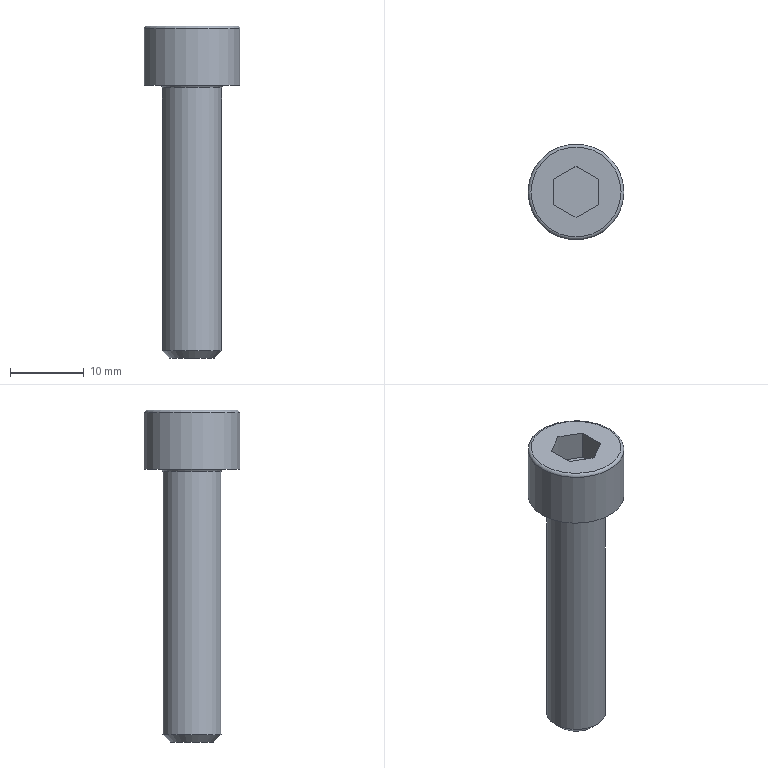Part | STEP file | solid 161 | 1 solid | 15 faces | box 13 x 13 x 45 mm | volume 2785 mm3 | plane 10 | cylinder 2 | torus 2 | cone 1 | commonest cylinder face diameters 8 x1 13 x1